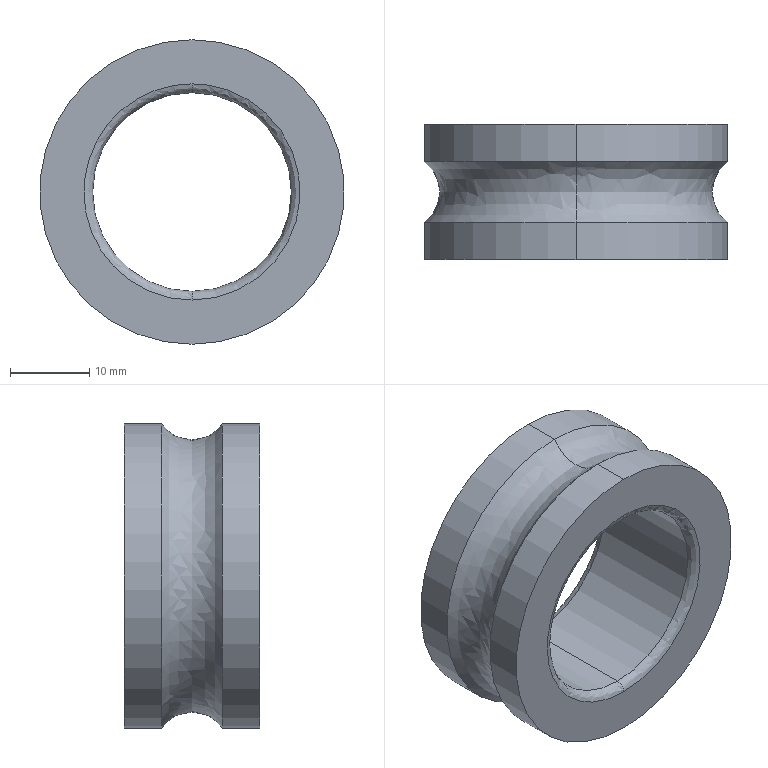Part | SolidWorks | features BaseBody 1 | 1 solid | 14 faces | box 38.32 x 17 x 38.32 mm | volume 9957 mm3 | spline 6 | cylinder 6 | plane 2 | commonest cylinder face diameters 38.32 x4 25 x2
STEP:
#1=CARTESIAN_POINT('',(0.,-7.4,12.5));
#2=VERTEX_POINT('',#1);
#3=CARTESIAN_POINT('',(0.,-7.4,-12.5));
#4=VERTEX_POINT('',#3);
#5=CARTESIAN_POINT('',(0.,-7.4,0.));
#6=DIRECTION('',(0.,1.,0.));
#7=DIRECTION('',(0.,0.,-1.));
#8=AXIS2_PLACEMENT_3D('',#5,#6,#7);
#9=CIRCLE('',#8,12.5);
#10=EDGE_CURVE('',#2,#4,#9,.T.);
#11=ORIENTED_EDGE('',*,*,#10,.T.);
#12=CARTESIAN_POINT('',(0.,-8.5,-13.6));
#13=VERTEX_POINT('',#12);
#14=CARTESIAN_POINT('',(0.,-7.4,-13.6));
#15=DIRECTION('',(1.,0.,0.));
#16=DIRECTION('',(0.,0.,-1.));
#17=AXIS2_PLACEMENT_3D('',#14,#15,#16);
#18=CIRCLE('',#17,1.1);
#19=EDGE_CURVE('',#4,#13,#18,.T.);
#20=ORIENTED_EDGE('',*,*,#19,.T.);
#21=CARTESIAN_POINT('',(0.,-8.5,13.6));
#22=VERTEX_POINT('',#21);
#23=CARTESIAN_POINT('',(0.,-8.5,-13.6));
#24=CARTESIAN_POINT('',(27.2,-8.5,-13.6));
#25=CARTESIAN_POINT('',(27.2,-8.5,13.6));
#26=CARTESIAN_POINT('',(0.,-8.5,13.6));
#27=(BOUNDED_CURVE()B_SPLINE_CURVE(3,(#23,#24,#25,#26),.UNSPECIFIED.,.F.,.F.)B_SPLINE_CURVE_WITH_KNOTS((4,4),(0.,1.),.UNSPECIFIED.)CURVE()GEOMETRIC_REPRESENTATION_ITEM()RATIONAL_B_SPLINE_CURVE((1.,0.3333,0.3333,1.))REPRESENTATION_ITEM(''));
#28=EDGE_CURVE('',#13,#22,#27,.T.);
#29=ORIENTED_EDGE('',*,*,#28,.T.);
#30=CARTESIAN_POINT('',(0.,-7.4,13.6));
#31=DIRECTION('',(-1.,0.,0.));
#32=DIRECTION('',(0.,0.,1.));
#33=AXIS2_PLACEMENT_3D('',#30,#31,#32);
#34=CIRCLE('',#33,1.1);
#35=EDGE_CURVE('',#2,#22,#34,.T.);
#36=ORIENTED_EDGE('',*,*,#35,.F.);
#37=EDGE_LOOP('',(#11,#20,#29,#36));
#38=FACE_OUTER_BOUND('',#37,.T.);
#39=CARTESIAN_POINT('',(0.,-7.4,-12.5));
#40=CARTESIAN_POINT('',(25.,-7.4,-12.5));
#41=CARTESIAN_POINT('',(25.,-7.4,12.5));
#42=CARTESIAN_POINT('',(0.,-7.4,12.5));
#43=CARTESIAN_POINT('',(0.,-8.044,-12.5));
#44=CARTESIAN_POINT('',(25.,-8.044,-12.5));
#45=CARTESIAN_POINT('',(25.,-8.044,12.5));
#46=CARTESIAN_POINT('',(0.,-8.044,12.5));
#47=CARTESIAN_POINT('',(0.,-8.5,-12.956));
#48=CARTESIAN_POINT('',(25.911,-8.5,-12.956));
#49=CARTESIAN_POINT('',(25.911,-8.5,12.956));
#50=CARTESIAN_POINT('',(0.,-8.5,12.956));
#51=CARTESIAN_POINT('',(0.,-8.5,-13.6));
#52=CARTESIAN_POINT('',(27.2,-8.5,-13.6));
#53=CARTESIAN_POINT('',(27.2,-8.5,13.6));
#54=CARTESIAN_POINT('',(0.,-8.5,13.6));
#55=(BOUNDED_SURFACE()B_SPLINE_SURFACE(3,3,((#39,#40,#41,#42),(#43,#44,#45,#46),(#47,#48,#49,#50),(#51,#52,#53,#54)),.UNSPECIFIED.,.F.,.F.,.F.)B_SPLINE_SURFACE_WITH_KNOTS((4,4),(4,4),(0.,1.),(0.,1.),.UNSPECIFIED.)GEOMETRIC_REPRESENTATION_ITEM()RATIONAL_B_SPLINE_SURFACE(((1.,0.3333,0.3333,1.),(0.8047,0.2682,0.2682,0.8047),(0.8047,0.2682,0.2682,0.8047),(1.,0.3333,0.3333,1.)))REPRESENTATION_ITEM('')SURFACE());
#56=ADVANCED_FACE('',(#38),#55,.T.);
#57=CARTESIAN_POINT('',(0.,8.5,13.6));
#58=VERTEX_POINT('',#57);
#59=CARTESIAN_POINT('',(0.,8.5,-13.6));
#60=VERTEX_POINT('',#59);
#61=CARTESIAN_POINT('',(0.,8.5,13.6));
#62=CARTESIAN_POINT('',(27.2,8.5,13.6));
#63=CARTESIAN_POINT('',(27.2,8.5,-13.6));
#64=CARTESIAN_POINT('',(0.,8.5,-13.6));
#65=(BOUNDED_CURVE()B_SPLINE_CURVE(3,(#61,#62,#63,#64),.UNSPECIFIED.,.F.,.F.)B_SPLINE_CURVE_WITH_KNOTS((4,4),(0.,1.),.UNSPECIFIED.)CURVE()GEOMETRIC_REPRESENTATION_ITEM()RATIONAL_B_SPLINE_CURVE((1.,0.3333,0.3333,1.))REPRESENTATION_ITEM(''));
#66=EDGE_CURVE('',#58,#60,#65,.T.);
#67=ORIENTED_EDGE('',*,*,#66,.T.);
#68=CARTESIAN_POINT('',(0.,7.4,-12.5));
#69=VERTEX_POINT('',#68);
#70=CARTESIAN_POINT('',(0.,7.4,-13.6));
#71=DIRECTION('',(1.,0.,0.));
#72=DIRECTION('',(0.,0.,-1.));
#73=AXIS2_PLACEMENT_3D('',#70,#71,#72);
#74=CIRCLE('',#73,1.1);
#75=EDGE_CURVE('',#60,#69,#74,.T.);
#76=ORIENTED_EDGE('',*,*,#75,.T.);
#77=CARTESIAN_POINT('',(0.,7.4,12.5));
#78=VERTEX_POINT('',#77);
#79=CARTESIAN_POINT('',(0.,7.4,0.));
#80=DIRECTION('',(0.,-1.,0.));
#81=DIRECTION('',(0.,0.,-1.));
#82=AXIS2_PLACEMENT_3D('',#79,#80,#81);
#83=CIRCLE('',#82,12.5);
#84=EDGE_CURVE('',#69,#78,#83,.T.);
#85=ORIENTED_EDGE('',*,*,#84,.T.);
#86=CARTESIAN_POINT('',(0.,7.4,13.6));
#87=DIRECTION('',(-1.,0.,0.));
#88=DIRECTION('',(0.,0.,1.));
#89=AXIS2_PLACEMENT_3D('',#86,#87,#88);
#90=CIRCLE('',#89,1.1);
#91=EDGE_CURVE('',#58,#78,#90,.T.);
#92=ORIENTED_EDGE('',*,*,#91,.F.);
#93=EDGE_LOOP('',(#67,#76,#85,#92));
#94=FACE_OUTER_BOUND('',#93,.T.);
#95=CARTESIAN_POINT('',(0.,8.5,-13.6));
#96=CARTESIAN_POINT('',(27.2,8.5,-13.6));
#97=CARTESIAN_POINT('',(27.2,8.5,13.6));
#98=CARTESIAN_POINT('',(0.,8.5,13.6));
#99=CARTESIAN_POINT('',(0.,8.5,-12.956));
#100=CARTESIAN_POINT('',(25.911,8.5,-12.956));
#101=CARTESIAN_POINT('',(25.911,8.5,12.956));
#102=CARTESIAN_POINT('',(0.,8.5,12.956));
#103=CARTESIAN_POINT('',(0.,8.044,-12.5));
#104=CARTESIAN_POINT('',(25.,8.044,-12.5));
#105=CARTESIAN_POINT('',(25.,8.044,12.5));
#106=CARTESIAN_POINT('',(0.,8.044,12.5));
#107=CARTESIAN_POINT('',(0.,7.4,-12.5));
#108=CARTESIAN_POINT('',(25.,7.4,-12.5));
#109=CARTESIAN_POINT('',(25.,7.4,12.5));
#110=CARTESIAN_POINT('',(0.,7.4,12.5));
#111=(BOUNDED_SURFACE()B_SPLINE_SURFACE(3,3,((#95,#96,#97,#98),(#99,#100,#101,#102),(#103,#104,#105,#106),(#107,#108,#109,#110)),.UNSPECIFIED.,.F.,.F.,.F.)B_SPLINE_SURFACE_WITH_KNOTS((4,4),(4,4),(0.,1.),(0.,1.),.UNSPECIFIED.)GEOMETRIC_REPRESENTATION_ITEM()RATIONAL_B_SPLINE_SURFACE(((1.,0.3333,0.3333,1.),(0.8047,0.2682,0.2682,0.8047),(0.8047,0.2682,0.2682,0.8047),(1.,0.3333,0.3333,1.)))REPRESENTATION_ITEM('')SURFACE());
#112=ADVANCED_FACE('',(#94),#111,.T.);
#113=CARTESIAN_POINT('',(0.,3.832,-19.16));
#114=VERTEX_POINT('',#113);
#115=CARTESIAN_POINT('',(0.,3.832,19.16));
#116=VERTEX_POINT('',#115);
#117=CARTESIAN_POINT('',(0.,3.832,0.));
#118=DIRECTION('',(0.,1.,0.));
#119=DIRECTION('',(0.,0.,-1.));
#120=AXIS2_PLACEMENT_3D('',#117,#118,#119);
#121=CIRCLE('',#120,19.16);
#122=EDGE_CURVE('',#114,#116,#121,.T.);
#123=ORIENTED_EDGE('',*,*,#122,.F.);
#124=CARTESIAN_POINT('',(0.,-3.832,-19.16));
#125=VERTEX_POINT('',#124);
#126=CARTESIAN_POINT('',(0.,0.,-21.75));
#127=DIRECTION('',(1.,0.,0.));
#128=DIRECTION('',(0.,0.,-1.));
#129=AXIS2_PLACEMENT_3D('',#126,#127,#128);
#130=CIRCLE('',#129,4.625);
#131=EDGE_CURVE('',#114,#125,#130,.T.);
#132=ORIENTED_EDGE('',*,*,#131,.T.);
#133=CARTESIAN_POINT('',(0.,-3.832,19.16));
#134=VERTEX_POINT('',#133);
#135=CARTESIAN_POINT('',(0.,-3.832,0.));
#136=DIRECTION('',(0.,-1.,0.));
#137=DIRECTION('',(0.,0.,-1.));
#138=AXIS2_PLACEMENT_3D('',#135,#136,#137);
#139=CIRCLE('',#138,19.16);
#140=EDGE_CURVE('',#134,#125,#139,.T.);
#141=ORIENTED_EDGE('',*,*,#140,.F.);
#142=CARTESIAN_POINT('',(0.,0.,21.75));
#143=DIRECTION('',(-1.,0.,0.));
#144=DIRECTION('',(0.,0.,1.));
#145=AXIS2_PLACEMENT_3D('',#142,#143,#144);
#146=CIRCLE('',#145,4.625);
#147=EDGE_CURVE('',#116,#134,#146,.T.);
#148=ORIENTED_EDGE('',*,*,#147,.F.);
#149=EDGE_LOOP('',(#123,#132,#141,#148));
#150=FACE_OUTER_BOUND('',#149,.T.);
#151=CARTESIAN_POINT('',(0.,3.832,19.16));
#152=CARTESIAN_POINT('',(-38.32,3.832,19.16));
#153=CARTESIAN_POINT('',(-38.32,3.832,-19.16));
#154=CARTESIAN_POINT('',(0.,3.832,-19.16));
#155=CARTESIAN_POINT('',(0.,1.807,16.165));
#156=CARTESIAN_POINT('',(-32.33,1.807,16.165));
#157=CARTESIAN_POINT('',(-32.33,1.807,-16.165));
#158=CARTESIAN_POINT('',(0.,1.807,-16.165));
#159=CARTESIAN_POINT('',(0.,-1.807,16.165));
#160=CARTESIAN_POINT('',(-32.33,-1.807,16.165));
#161=CARTESIAN_POINT('',(-32.33,-1.807,-16.165));
#162=CARTESIAN_POINT('',(0.,-1.807,-16.165));
#163=CARTESIAN_POINT('',(0.,-3.832,19.16));
#164=CARTESIAN_POINT('',(-38.32,-3.832,19.16));
#165=CARTESIAN_POINT('',(-38.32,-3.832,-19.16));
#166=CARTESIAN_POINT('',(0.,-3.832,-19.16));
#167=(BOUNDED_SURFACE()B_SPLINE_SURFACE(3,3,((#151,#152,#153,#154),(#155,#156,#157,#158),(#159,#160,#161,#162),(#163,#164,#165,#166)),.UNSPECIFIED.,.F.,.F.,.F.)B_SPLINE_SURFACE_WITH_KNOTS((4,4),(4,4),(0.,1.),(0.,1.),.UNSPECIFIED.)GEOMETRIC_REPRESENTATION_ITEM()RATIONAL_B_SPLINE_SURFACE(((1.,0.3333,0.3333,1.),(0.7067,0.2356,0.2356,0.7067),(0.7067,0.2356,0.2356,0.7067),(1.,0.3333,0.3333,1.)))REPRESENTATION_ITEM('')SURFACE());
#168=ADVANCED_FACE('',(#150),#167,.F.);
#169=CARTESIAN_POINT('',(0.,7.4,0.));
#170=DIRECTION('',(0.,-1.,0.));
#171=DIRECTION('',(0.,0.,-1.));
#172=AXIS2_PLACEMENT_3D('',#169,#170,#171);
#173=CIRCLE('',#172,12.5);
#174=EDGE_CURVE('',#78,#69,#173,.T.);
#175=ORIENTED_EDGE('',*,*,#174,.F.);
#176=CARTESIAN_POINT('',(0.,9.35,12.5));
#177=DIRECTION('',(0.,-1.,0.));
#178=VECTOR('',#177,1000.);
#179=LINE('',#176,#178);
#180=EDGE_CURVE('',#78,#2,#179,.T.);
#181=ORIENTED_EDGE('',*,*,#180,.T.);
#182=CARTESIAN_POINT('',(0.,-7.4,0.));
#183=DIRECTION('',(0.,1.,0.));
#184=DIRECTION('',(0.,0.,-1.));
#185=AXIS2_PLACEMENT_3D('',#182,#183,#184);
#186=CIRCLE('',#185,12.5);
#187=EDGE_CURVE('',#4,#2,#186,.T.);
#188=ORIENTED_EDGE('',*,*,#187,.F.);
#189=CARTESIAN_POINT('',(0.,9.35,-12.5));
#190=DIRECTION('',(0.,-1.,0.));
#191=VECTOR('',#190,1000.);
#192=LINE('',#189,#191);
#193=EDGE_CURVE('',#69,#4,#192,.T.);
#194=ORIENTED_EDGE('',*,*,#193,.F.);
#195=EDGE_LOOP('',(#175,#181,#188,#194));
#196=FACE_OUTER_BOUND('',#195,.T.);
#197=CARTESIAN_POINT('',(0.,9.35,0.));
#198=DIRECTION('',(0.,-1.,0.));
#199=DIRECTION('',(0.,0.,-1.));
#200=AXIS2_PLACEMENT_3D('',#197,#198,#199);
#201=CYLINDRICAL_SURFACE('',#200,12.5);
#202=ADVANCED_FACE('',(#196),#201,.F.);
#203=CARTESIAN_POINT('',(0.,-3.832,0.));
#204=DIRECTION('',(0.,-1.,0.));
#205=DIRECTION('',(0.,0.,-1.));
#206=AXIS2_PLACEMENT_3D('',#203,#204,#205);
#207=CIRCLE('',#206,19.16);
#208=EDGE_CURVE('',#125,#134,#207,.T.);
#209=ORIENTED_EDGE('',*,*,#208,.T.);
#210=CARTESIAN_POINT('',(0.,-8.5,19.16));
#211=VERTEX_POINT('',#210);
#212=CARTESIAN_POINT('',(0.,9.35,19.16));
#213=DIRECTION('',(0.,-1.,0.));
#214=VECTOR('',#213,1000.);
#215=LINE('',#212,#214);
#216=EDGE_CURVE('',#134,#211,#215,.T.);
#217=ORIENTED_EDGE('',*,*,#216,.T.);
#218=CARTESIAN_POINT('',(0.,-8.5,-19.16));
#219=VERTEX_POINT('',#218);
#220=CARTESIAN_POINT('',(0.,-8.5,0.));
#221=DIRECTION('',(0.,-1.,0.));
#222=DIRECTION('',(0.,0.,-1.));
#223=AXIS2_PLACEMENT_3D('',#220,#221,#222);
#224=CIRCLE('',#223,19.16);
#225=EDGE_CURVE('',#219,#211,#224,.T.);
#226=ORIENTED_EDGE('',*,*,#225,.F.);
#227=CARTESIAN_POINT('',(0.,9.35,-19.16));
#228=DIRECTION('',(0.,-1.,0.));
#229=VECTOR('',#228,1000.);
#230=LINE('',#227,#229);
#231=EDGE_CURVE('',#125,#219,#230,.T.);
#232=ORIENTED_EDGE('',*,*,#231,.F.);
#233=EDGE_LOOP('',(#209,#217,#226,#232));
#234=FACE_OUTER_BOUND('',#233,.T.);
#235=CARTESIAN_POINT('',(0.,9.35,0.));
#236=DIRECTION('',(0.,-1.,0.));
#237=DIRECTION('',(0.,0.,-1.));
#238=AXIS2_PLACEMENT_3D('',#235,#236,#237);
#239=CYLINDRICAL_SURFACE('',#238,19.16);
#240=ADVANCED_FACE('',(#234),#239,.T.);
#241=CARTESIAN_POINT('',(0.,8.5,-19.16));
#242=VERTEX_POINT('',#241);
#243=CARTESIAN_POINT('',(0.,8.5,19.16));
#244=VERTEX_POINT('',#243);
#245=CARTESIAN_POINT('',(0.,8.5,0.));
#246=DIRECTION('',(0.,-1.,0.));
#247=DIRECTION('',(0.,0.,-1.));
#248=AXIS2_PLACEMENT_3D('',#245,#246,#247);
#249=CIRCLE('',#248,19.16);
#250=EDGE_CURVE('',#242,#244,#249,.T.);
#251=ORIENTED_EDGE('',*,*,#250,.T.);
#252=CARTESIAN_POINT('',(0.,9.35,19.16));
#253=DIRECTION('',(0.,-1.,0.));
#254=VECTOR('',#253,1000.);
#255=LINE('',#252,#254);
#256=EDGE_CURVE('',#244,#116,#255,.T.);
#257=ORIENTED_EDGE('',*,*,#256,.T.);
#258=CARTESIAN_POINT('',(0.,3.832,0.));
#259=DIRECTION('',(0.,1.,0.));
#260=DIRECTION('',(0.,0.,-1.));
#261=AXIS2_PLACEMENT_3D('',#258,#259,#260);
#262=CIRCLE('',#261,19.16);
#263=EDGE_CURVE('',#116,#114,#262,.T.);
#264=ORIENTED_EDGE('',*,*,#263,.T.);
#265=CARTESIAN_POINT('',(0.,9.35,-19.16));
#266=DIRECTION('',(0.,-1.,0.));
#267=VECTOR('',#266,1000.);
#268=LINE('',#265,#267);
#269=EDGE_CURVE('',#242,#114,#268,.T.);
#270=ORIENTED_EDGE('',*,*,#269,.F.);
#271=EDGE_LOOP('',(#251,#257,#264,#270));
#272=FACE_OUTER_BOUND('',#271,.T.);
#273=CARTESIAN_POINT('',(0.,9.35,0.));
#274=DIRECTION('',(0.,-1.,0.));
#275=DIRECTION('',(0.,0.,-1.));
#276=AXIS2_PLACEMENT_3D('',#273,#274,#275);
#277=CYLINDRICAL_SURFACE('',#276,19.16);
#278=ADVANCED_FACE('',(#272),#277,.T.);
#279=ORIENTED_EDGE('',*,*,#180,.F.);
#280=ORIENTED_EDGE('',*,*,#84,.F.);
#281=ORIENTED_EDGE('',*,*,#193,.T.);
#282=ORIENTED_EDGE('',*,*,#10,.F.);
#283=EDGE_LOOP('',(#279,#280,#281,#282));
#284=FACE_OUTER_BOUND('',#283,.T.);
#285=CARTESIAN_POINT('',(0.,9.35,0.));
#286=DIRECTION('',(0.,-1.,0.));
#287=DIRECTION('',(0.,0.,-1.));
#288=AXIS2_PLACEMENT_3D('',#285,#286,#287);
#289=CYLINDRICAL_SURFACE('',#288,12.5);
#290=ADVANCED_FACE('',(#284),#289,.F.);
#291=ORIENTED_EDGE('',*,*,#19,.F.);
#292=ORIENTED_EDGE('',*,*,#187,.T.);
#293=ORIENTED_EDGE('',*,*,#35,.T.);
#294=CARTESIAN_POINT('',(0.,-8.5,-13.6));
#295=CARTESIAN_POINT('',(-0.4158,-8.5,-13.6));
#296=CARTESIAN_POINT('',(-1.037,-8.5,-13.572));
#297=CARTESIAN_POINT('',(-1.757,-8.5,-13.489));
#298=CARTESIAN_POINT('',(-2.116,-8.5,-13.435));
#299=CARTESIAN_POINT('',(-2.296,-8.5,-13.405));
#300=CARTESIAN_POINT('',(-2.372,-8.5,-13.392));
#301=CARTESIAN_POINT('',(-2.424,-8.5,-13.382));
#302=CARTESIAN_POINT('',(-2.448,-8.5,-13.378));
#303=CARTESIAN_POINT('',(-2.908,-8.5,-13.293));
#304=CARTESIAN_POINT('',(-3.55,-8.5,-13.142));
#305=CARTESIAN_POINT('',(-4.283,-8.5,-12.911));
#306=CARTESIAN_POINT('',(-4.646,-8.5,-12.783));
#307=CARTESIAN_POINT('',(-4.826,-8.5,-12.715));
#308=CARTESIAN_POINT('',(-4.903,-8.5,-12.685));
#309=CARTESIAN_POINT('',(-4.955,-8.5,-12.665));
#310=CARTESIAN_POINT('',(-4.979,-8.5,-12.656));
#311=CARTESIAN_POINT('',(-5.433,-8.5,-12.476));
#312=CARTESIAN_POINT('',(-6.058,-8.5,-12.191));
#313=CARTESIAN_POINT('',(-6.759,-8.5,-11.805));
#314=CARTESIAN_POINT('',(-7.103,-8.5,-11.599));
#315=CARTESIAN_POINT('',(-7.249,-8.5,-11.507));
#316=CARTESIAN_POINT('',(-7.346,-8.5,-11.446));
#317=CARTESIAN_POINT('',(-7.393,-8.5,-11.415));
#318=CARTESIAN_POINT('',(-8.228,-8.5,-10.87));
#319=CARTESIAN_POINT('',(-8.953,-8.5,-10.28));
#320=CARTESIAN_POINT('',(-9.948,-8.5,-9.285));
#321=CARTESIAN_POINT('',(-10.418,-8.5,-8.764));
#322=CARTESIAN_POINT('',(-10.917,-8.5,-8.117));
#323=CARTESIAN_POINT('',(-11.154,-8.5,-7.783));
#324=CARTESIAN_POINT('',(-11.253,-8.5,-7.637));
#325=CARTESIAN_POINT('',(-11.319,-8.5,-7.54));
#326=CARTESIAN_POINT('',(-11.352,-8.5,-7.49));
#327=CARTESIAN_POINT('',(-11.635,-8.5,-7.058));
#328=CARTESIAN_POINT('',(-11.981,-8.5,-6.465));
#329=CARTESIAN_POINT('',(-12.331,-8.5,-5.745));
#330=CARTESIAN_POINT('',(-12.493,-8.5,-5.378));
#331=CARTESIAN_POINT('',(-12.57,-8.5,-5.193));
#332=CARTESIAN_POINT('',(-12.602,-8.5,-5.113));
#333=CARTESIAN_POINT('',(-12.624,-8.5,-5.059));
#334=CARTESIAN_POINT('',(-12.635,-8.5,-5.032));
#335=CARTESIAN_POINT('',(-12.807,-8.5,-4.596));
#336=CARTESIAN_POINT('',(-13.02,-8.5,-3.972));
#337=CARTESIAN_POINT('',(-13.214,-8.5,-3.229));
#338=CARTESIAN_POINT('',(-13.298,-8.5,-2.853));
#339=CARTESIAN_POINT('',(-13.337,-8.5,-2.664));
#340=CARTESIAN_POINT('',(-13.352,-8.5,-2.583));
#341=CARTESIAN_POINT('',(-13.363,-8.5,-2.529));
#342=CARTESIAN_POINT('',(-13.368,-8.5,-2.5));
#343=CARTESIAN_POINT('',(-13.524,-8.5,-1.657));
#344=CARTESIAN_POINT('',(-13.6,-8.5,-0.8315));
#345=CARTESIAN_POINT('',(-13.6,-8.5,0.4157));
#346=CARTESIAN_POINT('',(-13.572,-8.5,1.037));
#347=CARTESIAN_POINT('',(-13.489,-8.5,1.757));
#348=CARTESIAN_POINT('',(-13.435,-8.5,2.116));
#349=CARTESIAN_POINT('',(-13.405,-8.5,2.296));
#350=CARTESIAN_POINT('',(-13.392,-8.5,2.372));
#351=CARTESIAN_POINT('',(-13.382,-8.5,2.424));
#352=CARTESIAN_POINT('',(-13.378,-8.5,2.448));
#353=CARTESIAN_POINT('',(-13.293,-8.5,2.908));
#354=CARTESIAN_POINT('',(-13.142,-8.5,3.55));
#355=CARTESIAN_POINT('',(-12.911,-8.5,4.283));
#356=CARTESIAN_POINT('',(-12.783,-8.5,4.646));
#357=CARTESIAN_POINT('',(-12.715,-8.5,4.826));
#358=CARTESIAN_POINT('',(-12.685,-8.5,4.903));
#359=CARTESIAN_POINT('',(-12.665,-8.5,4.955));
#360=CARTESIAN_POINT('',(-12.656,-8.5,4.979));
#361=CARTESIAN_POINT('',(-12.476,-8.5,5.433));
#362=CARTESIAN_POINT('',(-12.191,-8.5,6.058));
#363=CARTESIAN_POINT('',(-11.805,-8.5,6.759));
#364=CARTESIAN_POINT('',(-11.599,-8.5,7.103));
#365=CARTESIAN_POINT('',(-11.507,-8.5,7.249));
#366=CARTESIAN_POINT('',(-11.446,-8.5,7.346));
#367=CARTESIAN_POINT('',(-11.415,-8.5,7.393));
#368=CARTESIAN_POINT('',(-10.87,-8.5,8.228));
#369=CARTESIAN_POINT('',(-10.28,-8.5,8.953));
#370=CARTESIAN_POINT('',(-9.285,-8.5,9.948));
#371=CARTESIAN_POINT('',(-8.764,-8.5,10.418));
#372=CARTESIAN_POINT('',(-8.117,-8.5,10.917));
#373=CARTESIAN_POINT('',(-7.783,-8.5,11.154));
#374=CARTESIAN_POINT('',(-7.637,-8.5,11.253));
#375=CARTESIAN_POINT('',(-7.54,-8.5,11.319));
#376=CARTESIAN_POINT('',(-7.49,-8.5,11.352));
#377=CARTESIAN_POINT('',(-7.058,-8.5,11.635));
#378=CARTESIAN_POINT('',(-6.465,-8.5,11.981));
#379=CARTESIAN_POINT('',(-5.745,-8.5,12.331));
#380=CARTESIAN_POINT('',(-5.378,-8.5,12.493));
#381=CARTESIAN_POINT('',(-5.193,-8.5,12.57));
#382=CARTESIAN_POINT('',(-5.113,-8.5,12.602));
#383=CARTESIAN_POINT('',(-5.059,-8.5,12.624));
#384=CARTESIAN_POINT('',(-5.032,-8.5,12.635));
#385=CARTESIAN_POINT('',(-4.596,-8.5,12.807));
#386=CARTESIAN_POINT('',(-3.972,-8.5,13.02));
#387=CARTESIAN_POINT('',(-3.229,-8.5,13.214));
#388=CARTESIAN_POINT('',(-2.853,-8.5,13.298));
#389=CARTESIAN_POINT('',(-2.664,-8.5,13.337));
#390=CARTESIAN_POINT('',(-2.583,-8.5,13.352));
#391=CARTESIAN_POINT('',(-2.529,-8.5,13.363));
#392=CARTESIAN_POINT('',(-2.5,-8.5,13.368));
#393=CARTESIAN_POINT('',(-1.657,-8.5,13.524));
#394=CARTESIAN_POINT('',(-0.832,-8.5,13.6));
#395=CARTESIAN_POINT('',(0.,-8.5,13.6));
#396=B_SPLINE_CURVE_WITH_KNOTS('',3,(#294,#295,#296,#297,#298,#299,#300,#301,#302,#303,#304,#305,#306,#307,#308,#309,#310,#311,#312,#313,#314,#315,#316,#317,#318,#319,#320,#321,#322,#323,#324,#325,#326,#327,#328,#329,#330,#331,#332,#333,#334,#335,#336,#337,#338,#339,#340,#341,#342,#343,#344,#345,#346,#347,#348,#349,#350,#351,#352,#353,#354,#355,#356,#357,#358,#359,#360,#361,#362,#363,#364,#365,#366,#367,#368,#369,#370,#371,#372,#373,#374,#375,#376,#377,#378,#379,#380,#381,#382,#383,#384,#385,#386,#387,#388,#389,#390,#391,#392,#393,#394,#395),.UNSPECIFIED.,.F.,.F.,(4,1,1,1,1,2,2,1,1,1,1,2,2,1,1,1,2,2,2,1,1,1,2,2,1,1,1,1,2,2,1,1,1,1,2,2,2,1,1,1,1,2,2,1,1,1,1,2,2,1,1,1,2,2,2,1,1,1,2,2,1,1,1,1,2,2,1,1,1,1,2,2,4),(0.,0.03125,0.04687,0.05469,0.05859,0.06055,0.0625,0.09375,0.1094,0.1172,0.1211,0.123,0.125,0.1562,0.1719,0.1797,0.1836,0.1875,0.25,0.2812,0.2969,0.3047,0.3086,0.3125,0.3437,0.3594,0.3672,0.3711,0.373,0.375,0.4062,0.4219,0.4297,0.4336,0.4355,0.4375,0.5,0.5312,0.5469,0.5547,0.5586,0.5605,0.5625,0.5937,0.6094,0.6172,0.6211,0.623,0.625,0.6563,0.6719,0.6797,0.6836,0.6875,0.75,0.7813,0.7969,0.8047,0.8086,0.8125,0.8438,0.8594,0.8672,0.8711,0.873,0.875,0.9063,0.9219,0.9297,0.9336,0.9355,0.9375,1.),.UNSPECIFIED.);
#397=EDGE_CURVE('',#13,#22,#396,.T.);
#398=ORIENTED_EDGE('',*,*,#397,.F.);
#399=EDGE_LOOP('',(#291,#292,#293,#398));
#400=FACE_OUTER_BOUND('',#399,.T.);
#401=CARTESIAN_POINT('',(0.,-7.4,12.5));
#402=CARTESIAN_POINT('',(-25.,-7.4,12.5));
#403=CARTESIAN_POINT('',(-25.,-7.4,-12.5));
#404=CARTESIAN_POINT('',(0.,-7.4,-12.5));
#405=CARTESIAN_POINT('',(0.,-8.044,12.5));
#406=CARTESIAN_POINT('',(-25.,-8.044,12.5));
#407=CARTESIAN_POINT('',(-25.,-8.044,-12.5));
#408=CARTESIAN_POINT('',(0.,-8.044,-12.5));
#409=CARTESIAN_POINT('',(0.,-8.5,12.956));
#410=CARTESIAN_POINT('',(-25.911,-8.5,12.956));
#411=CARTESIAN_POINT('',(-25.911,-8.5,-12.956));
#412=CARTESIAN_POINT('',(0.,-8.5,-12.956));
#413=CARTESIAN_POINT('',(0.,-8.5,13.6));
#414=CARTESIAN_POINT('',(-27.2,-8.5,13.6));
#415=CARTESIAN_POINT('',(-27.2,-8.5,-13.6));
#416=CARTESIAN_POINT('',(0.,-8.5,-13.6));
#417=(BOUNDED_SURFACE()B_SPLINE_SURFACE(3,3,((#401,#402,#403,#404),(#405,#406,#407,#408),(#409,#410,#411,#412),(#413,#414,#415,#416)),.UNSPECIFIED.,.F.,.F.,.F.)B_SPLINE_SURFACE_WITH_KNOTS((4,4),(4,4),(0.,1.),(0.,1.),.UNSPECIFIED.)GEOMETRIC_REPRESENTATION_ITEM()RATIONAL_B_SPLINE_SURFACE(((1.,0.3333,0.3333,1.),(0.8047,0.2682,0.2682,0.8047),(0.8047,0.2682,0.2682,0.8047),(1.,0.3333,0.3333,1.)))REPRESENTATION_ITEM('')SURFACE());
#418=ADVANCED_FACE('',(#400),#417,.T.);
#419=ORIENTED_EDGE('',*,*,#75,.F.);
#420=CARTESIAN_POINT('',(0.,8.5,-13.6));
#421=CARTESIAN_POINT('',(-27.2,8.5,-13.6));
#422=CARTESIAN_POINT('',(-27.2,8.5,13.6));
#423=CARTESIAN_POINT('',(0.,8.5,13.6));
#424=(BOUNDED_CURVE()B_SPLINE_CURVE(3,(#420,#421,#422,#423),.UNSPECIFIED.,.F.,.F.)B_SPLINE_CURVE_WITH_KNOTS((4,4),(0.,1.),.UNSPECIFIED.)CURVE()GEOMETRIC_REPRESENTATION_ITEM()RATIONAL_B_SPLINE_CURVE((1.,0.3333,0.3333,1.))REPRESENTATION_ITEM(''));
#425=EDGE_CURVE('',#60,#58,#424,.T.);
#426=ORIENTED_EDGE('',*,*,#425,.T.);
#427=ORIENTED_EDGE('',*,*,#91,.T.);
#428=ORIENTED_EDGE('',*,*,#174,.T.);
#429=EDGE_LOOP('',(#419,#426,#427,#428));
#430=FACE_OUTER_BOUND('',#429,.T.);
#431=CARTESIAN_POINT('',(0.,8.5,13.6));
#432=CARTESIAN_POINT('',(-27.2,8.5,13.6));
#433=CARTESIAN_POINT('',(-27.2,8.5,-13.6));
#434=CARTESIAN_POINT('',(0.,8.5,-13.6));
#435=CARTESIAN_POINT('',(0.,8.5,12.956));
#436=CARTESIAN_POINT('',(-25.911,8.5,12.956));
#437=CARTESIAN_POINT('',(-25.911,8.5,-12.956));
#438=CARTESIAN_POINT('',(0.,8.5,-12.956));
#439=CARTESIAN_POINT('',(0.,8.044,12.5));
#440=CARTESIAN_POINT('',(-25.,8.044,12.5));
#441=CARTESIAN_POINT('',(-25.,8.044,-12.5));
#442=CARTESIAN_POINT('',(0.,8.044,-12.5));
#443=CARTESIAN_POINT('',(0.,7.4,12.5));
#444=CARTESIAN_POINT('',(-25.,7.4,12.5));
#445=CARTESIAN_POINT('',(-25.,7.4,-12.5));
#446=CARTESIAN_POINT('',(0.,7.4,-12.5));
#447=(BOUNDED_SURFACE()B_SPLINE_SURFACE(3,3,((#431,#432,#433,#434),(#435,#436,#437,#438),(#439,#440,#441,#442),(#443,#444,#445,#446)),.UNSPECIFIED.,.F.,.F.,.F.)B_SPLINE_SURFACE_WITH_KNOTS((4,4),(4,4),(0.,1.),(0.,1.),.UNSPECIFIED.)GEOMETRIC_REPRESENTATION_ITEM()RATIONAL_B_SPLINE_SURFACE(((1.,0.3333,0.3333,1.),(0.8047,0.2682,0.2682,0.8047),(0.8047,0.2682,0.2682,0.8047),(1.,0.3333,0.3333,1.)))REPRESENTATION_ITEM('')SURFACE());
#448=ADVANCED_FACE('',(#430),#447,.T.);
#449=ORIENTED_EDGE('',*,*,#28,.F.);
#450=ORIENTED_EDGE('',*,*,#397,.T.);
#451=EDGE_LOOP('',(#449,#450));
#452=FACE_BOUND('',#451,.T.);
#453=ORIENTED_EDGE('',*,*,#225,.T.);
#454=CARTESIAN_POINT('',(0.,-8.5,0.));
#455=DIRECTION('',(0.,-1.,0.));
#456=DIRECTION('',(0.,0.,-1.));
#457=AXIS2_PLACEMENT_3D('',#454,#455,#456);
#458=CIRCLE('',#457,19.16);
#459=EDGE_CURVE('',#211,#219,#458,.T.);
#460=ORIENTED_EDGE('',*,*,#459,.T.);
#461=EDGE_LOOP('',(#453,#460));
#462=FACE_OUTER_BOUND('',#461,.T.);
#463=CARTESIAN_POINT('',(0.,-8.5,0.));
#464=DIRECTION('',(0.,-1.,0.));
#465=DIRECTION('',(0.,0.,-1.));
#466=AXIS2_PLACEMENT_3D('',#463,#464,#465);
#467=PLANE('',#466);
#468=ADVANCED_FACE('',(#452,#462),#467,.T.);
#469=ORIENTED_EDGE('',*,*,#66,.F.);
#470=ORIENTED_EDGE('',*,*,#425,.F.);
#471=EDGE_LOOP('',(#469,#470));
#472=FACE_BOUND('',#471,.T.);
#473=ORIENTED_EDGE('',*,*,#250,.F.);
#474=CARTESIAN_POINT('',(0.,8.5,0.));
#475=DIRECTION('',(0.,-1.,0.));
#476=DIRECTION('',(0.,0.,-1.));
#477=AXIS2_PLACEMENT_3D('',#474,#475,#476);
#478=CIRCLE('',#477,19.16);
#479=EDGE_CURVE('',#244,#242,#478,.T.);
#480=ORIENTED_EDGE('',*,*,#479,.F.);
#481=EDGE_LOOP('',(#473,#480));
#482=FACE_OUTER_BOUND('',#481,.T.);
#483=CARTESIAN_POINT('',(0.,8.5,0.));
#484=DIRECTION('',(0.,-1.,0.));
#485=DIRECTION('',(0.,0.,-1.));
#486=AXIS2_PLACEMENT_3D('',#483,#484,#485);
#487=PLANE('',#486);
#488=ADVANCED_FACE('',(#472,#482),#487,.F.);
#489=ORIENTED_EDGE('',*,*,#216,.F.);
#490=ORIENTED_EDGE('',*,*,#140,.T.);
#491=ORIENTED_EDGE('',*,*,#231,.T.);
#492=ORIENTED_EDGE('',*,*,#459,.F.);
#493=EDGE_LOOP('',(#489,#490,#491,#492));
#494=FACE_OUTER_BOUND('',#493,.T.);
#495=CARTESIAN_POINT('',(0.,9.35,0.));
#496=DIRECTION('',(0.,-1.,0.));
#497=DIRECTION('',(0.,0.,-1.));
#498=AXIS2_PLACEMENT_3D('',#495,#496,#497);
#499=CYLINDRICAL_SURFACE('',#498,19.16);
#500=ADVANCED_FACE('',(#494),#499,.T.);
#501=ORIENTED_EDGE('',*,*,#256,.F.);
#502=ORIENTED_EDGE('',*,*,#479,.T.);
#503=ORIENTED_EDGE('',*,*,#269,.T.);
#504=ORIENTED_EDGE('',*,*,#122,.T.);
#505=EDGE_LOOP('',(#501,#502,#503,#504));
#506=FACE_OUTER_BOUND('',#505,.T.);
#507=CARTESIAN_POINT('',(0.,9.35,0.));
#508=DIRECTION('',(0.,-1.,0.));
#509=DIRECTION('',(0.,0.,-1.));
#510=AXIS2_PLACEMENT_3D('',#507,#508,#509);
#511=CYLINDRICAL_SURFACE('',#510,19.16);
#512=ADVANCED_FACE('',(#506),#511,.T.);
#513=ORIENTED_EDGE('',*,*,#131,.F.);
#514=ORIENTED_EDGE('',*,*,#263,.F.);
#515=ORIENTED_EDGE('',*,*,#147,.T.);
#516=ORIENTED_EDGE('',*,*,#208,.F.);
#517=EDGE_LOOP('',(#513,#514,#515,#516));
#518=FACE_OUTER_BOUND('',#517,.T.);
#519=CARTESIAN_POINT('',(0.,3.832,-19.16));
#520=CARTESIAN_POINT('',(38.32,3.832,-19.16));
#521=CARTESIAN_POINT('',(38.32,3.832,19.16));
#522=CARTESIAN_POINT('',(0.,3.832,19.16));
#523=CARTESIAN_POINT('',(0.,1.807,-16.165));
#524=CARTESIAN_POINT('',(32.33,1.807,-16.165));
#525=CARTESIAN_POINT('',(32.33,1.807,16.165));
#526=CARTESIAN_POINT('',(0.,1.807,16.165));
#527=CARTESIAN_POINT('',(0.,-1.807,-16.165));
#528=CARTESIAN_POINT('',(32.33,-1.807,-16.165));
#529=CARTESIAN_POINT('',(32.33,-1.807,16.165));
#530=CARTESIAN_POINT('',(0.,-1.807,16.165));
#531=CARTESIAN_POINT('',(0.,-3.832,-19.16));
#532=CARTESIAN_POINT('',(38.32,-3.832,-19.16));
#533=CARTESIAN_POINT('',(38.32,-3.832,19.16));
#534=CARTESIAN_POINT('',(0.,-3.832,19.16));
#535=(BOUNDED_SURFACE()B_SPLINE_SURFACE(3,3,((#519,#520,#521,#522),(#523,#524,#525,#526),(#527,#528,#529,#530),(#531,#532,#533,#534)),.UNSPECIFIED.,.F.,.F.,.F.)B_SPLINE_SURFACE_WITH_KNOTS((4,4),(4,4),(0.,1.),(0.,1.),.UNSPECIFIED.)GEOMETRIC_REPRESENTATION_ITEM()RATIONAL_B_SPLINE_SURFACE(((1.,0.3333,0.3333,1.),(0.7067,0.2356,0.2356,0.7067),(0.7067,0.2356,0.2356,0.7067),(1.,0.3333,0.3333,1.)))REPRESENTATION_ITEM('')SURFACE());
#536=ADVANCED_FACE('',(#518),#535,.F.);
#537=CLOSED_SHELL('',(#56,#112,#168,#202,#240,#278,#290,#418,#448,#468,#488,#500,#512,#536));
#538=MANIFOLD_SOLID_BREP('',#537);
#539=CARTESIAN_POINT('',(0.,0.,0.));
#540=DIRECTION('',(0.,0.,1.));
#541=DIRECTION('',(1.,0.,0.));
#542=AXIS2_PLACEMENT_3D('',#539,#540,#541);
#543=(LENGTH_UNIT()NAMED_UNIT(*)SI_UNIT(.MILLI.,.METRE.));
#544=UNCERTAINTY_MEASURE_WITH_UNIT(LENGTH_MEASURE(0.00001),#543,'','');
#545=(NAMED_UNIT(*)PLANE_ANGLE_UNIT()SI_UNIT($,.RADIAN.));
#546=(NAMED_UNIT(*)SI_UNIT($,.STERADIAN.)SOLID_ANGLE_UNIT());
#547=(GEOMETRIC_REPRESENTATION_CONTEXT(3)GLOBAL_UNCERTAINTY_ASSIGNED_CONTEXT((#544))GLOBAL_UNIT_ASSIGNED_CONTEXT((#543,#545,#546))REPRESENTATION_CONTEXT('',''));
#548=ADVANCED_BREP_SHAPE_REPRESENTATION('',(#538,#542),#547);